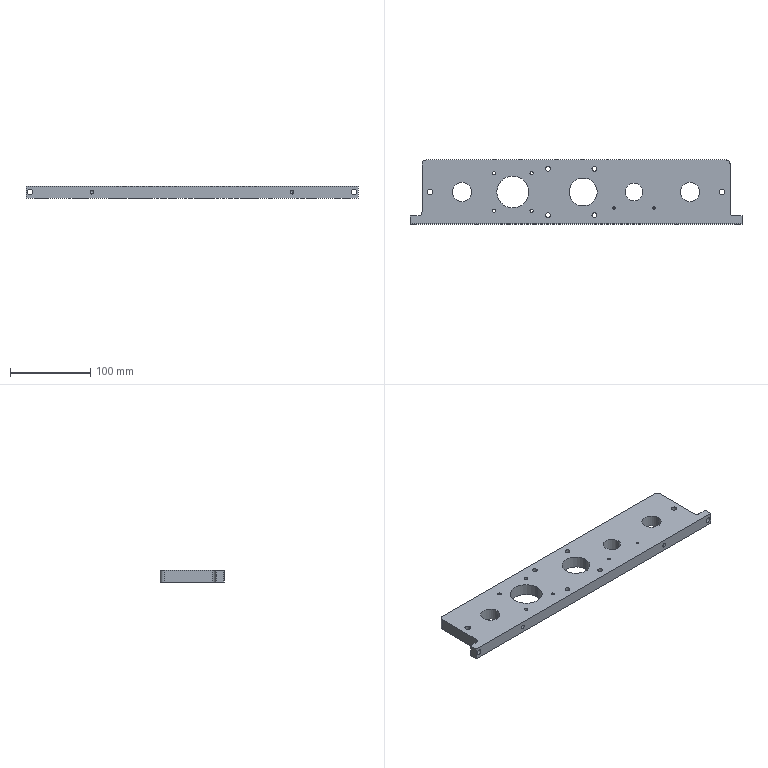Part | SolidWorks | features ICE 4, HoleWzd 3, Fillet 2, Extrusion 1 | 1 solid | 60 faces | box 415 x 80 x 15 mm | volume 408736 mm3 | cylinder 46 | plane 10 | cone 4 | commonest cylinder face diameters 4.2 x8 6 x8 6.8 x8 3.3 x4 5 x4 10 x4